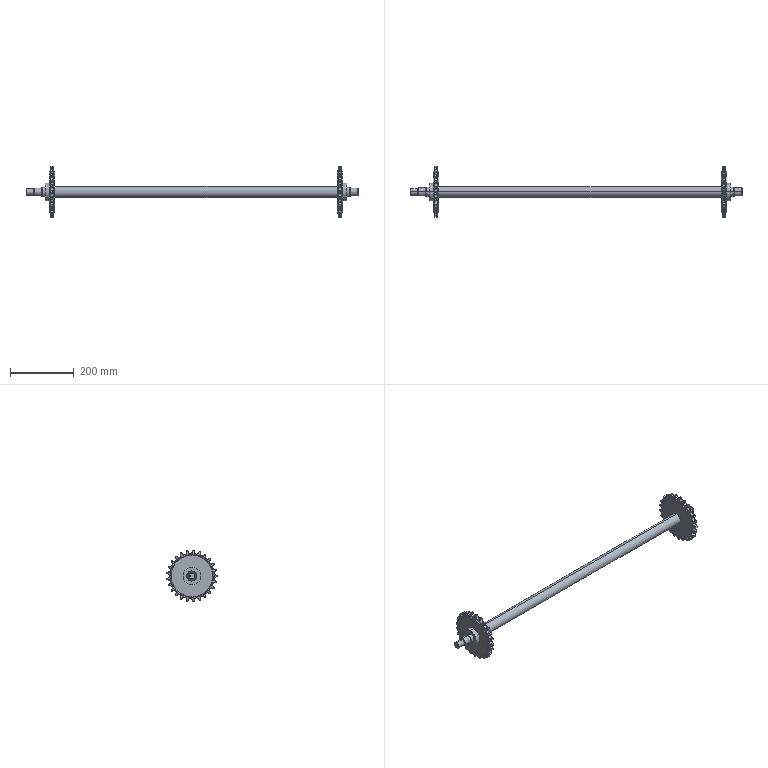Part | NX | features BREP 2 | 3 solids | 625 faces | box 1045 x 160.481 x 160.793 mm | volume 1442366 mm3 | cylinder 360 | plane 133 | torus 112 | cone 20 | commonest cylinder face diameters 17.202 x106 31.126 x104 12.07 x64 161 x50 30 x10 131 x8